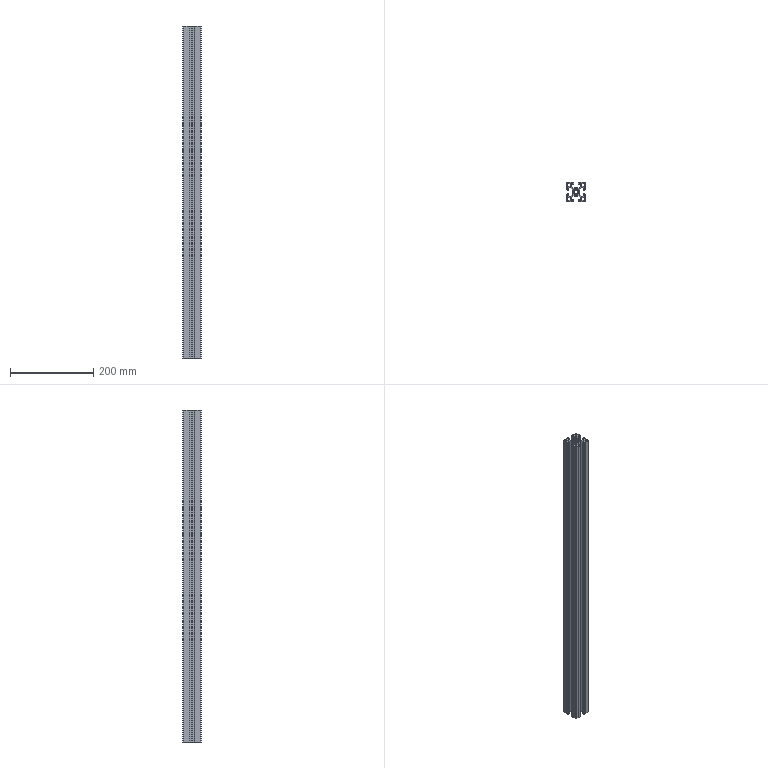Part | STEP file | PN_0017 | 1 solid | 271 faces | box 45 x 45 x 800 mm | volume 513293 mm3 | cylinder 149 | plane 122 | commonest cylinder face diameters 0.6 x48 1 x40 2 x28 10.2 x9 0.4 x8 16 x8